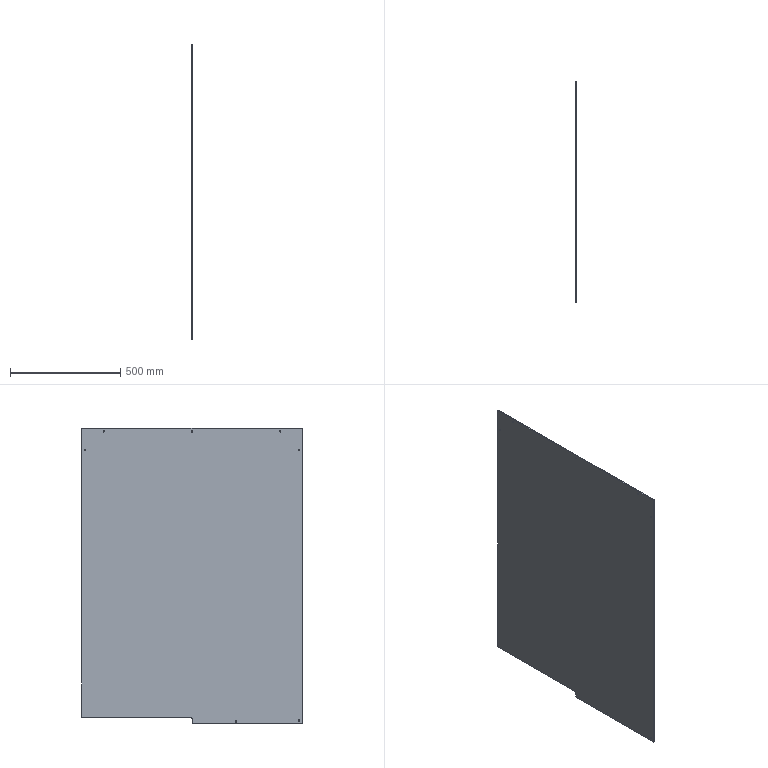Part | SolidWorks | features Chamfer 2, Fillet 2, ICE 2, Extrusion 1 | 1 solid | 28 faces | box 5 x 1000 x 1340 mm | volume 6624000 mm3 | cylinder 16 | plane 12 | commonest cylinder face diameters 6 x14 10 x2
STEP:
#1=CARTESIAN_POINT('',(5.,-200.,-662.));
#2=VERTEX_POINT('',#1);
#3=CARTESIAN_POINT('',(5.,-200.,-656.));
#4=VERTEX_POINT('',#3);
#5=CARTESIAN_POINT('',(5.,-200.,-659.));
#6=DIRECTION('',(-1.,0.,0.));
#7=DIRECTION('',(0.,0.,1.));
#8=AXIS2_PLACEMENT_3D('',#5,#6,#7);
#9=CIRCLE('',#8,3.);
#10=EDGE_CURVE('',#2,#4,#9,.T.);
#11=ORIENTED_EDGE('',*,*,#10,.F.);
#12=CARTESIAN_POINT('',(0.,-200.,-662.));
#13=VERTEX_POINT('',#12);
#14=CARTESIAN_POINT('',(5.,-200.,-662.));
#15=DIRECTION('',(-1.,0.,0.));
#16=VECTOR('',#15,1000.);
#17=LINE('',#14,#16);
#18=EDGE_CURVE('',#2,#13,#17,.T.);
#19=ORIENTED_EDGE('',*,*,#18,.T.);
#20=CARTESIAN_POINT('',(0.,-200.,-656.));
#21=VERTEX_POINT('',#20);
#22=CARTESIAN_POINT('',(0.,-200.,-659.));
#23=DIRECTION('',(-1.,0.,0.));
#24=DIRECTION('',(0.,0.,1.));
#25=AXIS2_PLACEMENT_3D('',#22,#23,#24);
#26=CIRCLE('',#25,3.);
#27=EDGE_CURVE('',#13,#21,#26,.T.);
#28=ORIENTED_EDGE('',*,*,#27,.T.);
#29=CARTESIAN_POINT('',(5.,-200.,-656.));
#30=DIRECTION('',(-1.,0.,0.));
#31=VECTOR('',#30,1000.);
#32=LINE('',#29,#31);
#33=EDGE_CURVE('',#4,#21,#32,.T.);
#34=ORIENTED_EDGE('',*,*,#33,.F.);
#35=EDGE_LOOP('',(#11,#19,#28,#34));
#36=FACE_OUTER_BOUND('',#35,.T.);
#37=CARTESIAN_POINT('',(5.,-200.,-659.));
#38=DIRECTION('',(-1.,0.,0.));
#39=DIRECTION('',(0.,0.,1.));
#40=AXIS2_PLACEMENT_3D('',#37,#38,#39);
#41=CYLINDRICAL_SURFACE('',#40,3.);
#42=ADVANCED_FACE('',(#36),#41,.F.);
#43=CARTESIAN_POINT('',(5.,0.,652.));
#44=VERTEX_POINT('',#43);
#45=CARTESIAN_POINT('',(5.,0.,658.));
#46=VERTEX_POINT('',#45);
#47=CARTESIAN_POINT('',(5.,0.,655.));
#48=DIRECTION('',(-1.,0.,0.));
#49=DIRECTION('',(0.,0.,1.));
#50=AXIS2_PLACEMENT_3D('',#47,#48,#49);
#51=CIRCLE('',#50,3.);
#52=EDGE_CURVE('',#44,#46,#51,.T.);
#53=ORIENTED_EDGE('',*,*,#52,.F.);
#54=CARTESIAN_POINT('',(0.,0.,652.));
#55=VERTEX_POINT('',#54);
#56=CARTESIAN_POINT('',(5.,0.,652.));
#57=DIRECTION('',(-1.,0.,0.));
#58=VECTOR('',#57,1000.);
#59=LINE('',#56,#58);
#60=EDGE_CURVE('',#44,#55,#59,.T.);
#61=ORIENTED_EDGE('',*,*,#60,.T.);
#62=CARTESIAN_POINT('',(0.,0.,658.));
#63=VERTEX_POINT('',#62);
#64=CARTESIAN_POINT('',(0.,0.,655.));
#65=DIRECTION('',(-1.,0.,0.));
#66=DIRECTION('',(0.,0.,1.));
#67=AXIS2_PLACEMENT_3D('',#64,#65,#66);
#68=CIRCLE('',#67,3.);
#69=EDGE_CURVE('',#55,#63,#68,.T.);
#70=ORIENTED_EDGE('',*,*,#69,.T.);
#71=CARTESIAN_POINT('',(5.,0.,658.));
#72=DIRECTION('',(-1.,0.,0.));
#73=VECTOR('',#72,1000.);
#74=LINE('',#71,#73);
#75=EDGE_CURVE('',#46,#63,#74,.T.);
#76=ORIENTED_EDGE('',*,*,#75,.F.);
#77=EDGE_LOOP('',(#53,#61,#70,#76));
#78=FACE_OUTER_BOUND('',#77,.T.);
#79=CARTESIAN_POINT('',(5.,0.,655.));
#80=DIRECTION('',(-1.,0.,0.));
#81=DIRECTION('',(0.,0.,1.));
#82=AXIS2_PLACEMENT_3D('',#79,#80,#81);
#83=CYLINDRICAL_SURFACE('',#82,3.);
#84=ADVANCED_FACE('',(#78),#83,.F.);
#85=CARTESIAN_POINT('',(5.,-485.,567.));
#86=VERTEX_POINT('',#85);
#87=CARTESIAN_POINT('',(5.,-485.,573.));
#88=VERTEX_POINT('',#87);
#89=CARTESIAN_POINT('',(5.,-485.,570.));
#90=DIRECTION('',(-1.,0.,0.));
#91=DIRECTION('',(0.,0.,1.));
#92=AXIS2_PLACEMENT_3D('',#89,#90,#91);
#93=CIRCLE('',#92,3.);
#94=EDGE_CURVE('',#86,#88,#93,.T.);
#95=ORIENTED_EDGE('',*,*,#94,.F.);
#96=CARTESIAN_POINT('',(0.,-485.,567.));
#97=VERTEX_POINT('',#96);
#98=CARTESIAN_POINT('',(5.,-485.,567.));
#99=DIRECTION('',(-1.,0.,0.));
#100=VECTOR('',#99,1000.);
#101=LINE('',#98,#100);
#102=EDGE_CURVE('',#86,#97,#101,.T.);
#103=ORIENTED_EDGE('',*,*,#102,.T.);
#104=CARTESIAN_POINT('',(0.,-485.,573.));
#105=VERTEX_POINT('',#104);
#106=CARTESIAN_POINT('',(0.,-485.,570.));
#107=DIRECTION('',(-1.,0.,0.));
#108=DIRECTION('',(0.,0.,1.));
#109=AXIS2_PLACEMENT_3D('',#106,#107,#108);
#110=CIRCLE('',#109,3.);
#111=EDGE_CURVE('',#97,#105,#110,.T.);
#112=ORIENTED_EDGE('',*,*,#111,.T.);
#113=CARTESIAN_POINT('',(5.,-485.,573.));
#114=DIRECTION('',(-1.,0.,0.));
#115=VECTOR('',#114,1000.);
#116=LINE('',#113,#115);
#117=EDGE_CURVE('',#88,#105,#116,.T.);
#118=ORIENTED_EDGE('',*,*,#117,.F.);
#119=EDGE_LOOP('',(#95,#103,#112,#118));
#120=FACE_OUTER_BOUND('',#119,.T.);
#121=CARTESIAN_POINT('',(5.,-485.,570.));
#122=DIRECTION('',(-1.,0.,0.));
#123=DIRECTION('',(0.,0.,1.));
#124=AXIS2_PLACEMENT_3D('',#121,#122,#123);
#125=CYLINDRICAL_SURFACE('',#124,3.);
#126=ADVANCED_FACE('',(#120),#125,.F.);
#127=CARTESIAN_POINT('',(5.,-400.,652.));
#128=VERTEX_POINT('',#127);
#129=CARTESIAN_POINT('',(5.,-400.,658.));
#130=VERTEX_POINT('',#129);
#131=CARTESIAN_POINT('',(5.,-400.,655.));
#132=DIRECTION('',(-1.,0.,0.));
#133=DIRECTION('',(0.,0.,1.));
#134=AXIS2_PLACEMENT_3D('',#131,#132,#133);
#135=CIRCLE('',#134,3.);
#136=EDGE_CURVE('',#128,#130,#135,.T.);
#137=ORIENTED_EDGE('',*,*,#136,.F.);
#138=CARTESIAN_POINT('',(0.,-400.,652.));
#139=VERTEX_POINT('',#138);
#140=CARTESIAN_POINT('',(5.,-400.,652.));
#141=DIRECTION('',(-1.,0.,0.));
#142=VECTOR('',#141,1000.);
#143=LINE('',#140,#142);
#144=EDGE_CURVE('',#128,#139,#143,.T.);
#145=ORIENTED_EDGE('',*,*,#144,.T.);
#146=CARTESIAN_POINT('',(0.,-400.,658.));
#147=VERTEX_POINT('',#146);
#148=CARTESIAN_POINT('',(0.,-400.,655.));
#149=DIRECTION('',(-1.,0.,0.));
#150=DIRECTION('',(0.,0.,1.));
#151=AXIS2_PLACEMENT_3D('',#148,#149,#150);
#152=CIRCLE('',#151,3.);
#153=EDGE_CURVE('',#139,#147,#152,.T.);
#154=ORIENTED_EDGE('',*,*,#153,.T.);
#155=CARTESIAN_POINT('',(5.,-400.,658.));
#156=DIRECTION('',(-1.,0.,0.));
#157=VECTOR('',#156,1000.);
#158=LINE('',#155,#157);
#159=EDGE_CURVE('',#130,#147,#158,.T.);
#160=ORIENTED_EDGE('',*,*,#159,.F.);
#161=EDGE_LOOP('',(#137,#145,#154,#160));
#162=FACE_OUTER_BOUND('',#161,.T.);
#163=CARTESIAN_POINT('',(5.,-400.,655.));
#164=DIRECTION('',(-1.,0.,0.));
#165=DIRECTION('',(0.,0.,1.));
#166=AXIS2_PLACEMENT_3D('',#163,#164,#165);
#167=CYLINDRICAL_SURFACE('',#166,3.);
#168=ADVANCED_FACE('',(#162),#167,.F.);
#169=CARTESIAN_POINT('',(5.,400.,652.));
#170=VERTEX_POINT('',#169);
#171=CARTESIAN_POINT('',(5.,400.,658.));
#172=VERTEX_POINT('',#171);
#173=CARTESIAN_POINT('',(5.,400.,655.));
#174=DIRECTION('',(-1.,0.,0.));
#175=DIRECTION('',(0.,0.,1.));
#176=AXIS2_PLACEMENT_3D('',#173,#174,#175);
#177=CIRCLE('',#176,3.);
#178=EDGE_CURVE('',#170,#172,#177,.T.);
#179=ORIENTED_EDGE('',*,*,#178,.F.);
#180=CARTESIAN_POINT('',(0.,400.,652.));
#181=VERTEX_POINT('',#180);
#182=CARTESIAN_POINT('',(5.,400.,652.));
#183=DIRECTION('',(-1.,0.,0.));
#184=VECTOR('',#183,1000.);
#185=LINE('',#182,#184);
#186=EDGE_CURVE('',#170,#181,#185,.T.);
#187=ORIENTED_EDGE('',*,*,#186,.T.);
#188=CARTESIAN_POINT('',(0.,400.,658.));
#189=VERTEX_POINT('',#188);
#190=CARTESIAN_POINT('',(0.,400.,655.));
#191=DIRECTION('',(-1.,0.,0.));
#192=DIRECTION('',(0.,0.,1.));
#193=AXIS2_PLACEMENT_3D('',#190,#191,#192);
#194=CIRCLE('',#193,3.);
#195=EDGE_CURVE('',#181,#189,#194,.T.);
#196=ORIENTED_EDGE('',*,*,#195,.T.);
#197=CARTESIAN_POINT('',(5.,400.,658.));
#198=DIRECTION('',(-1.,0.,0.));
#199=VECTOR('',#198,1000.);
#200=LINE('',#197,#199);
#201=EDGE_CURVE('',#172,#189,#200,.T.);
#202=ORIENTED_EDGE('',*,*,#201,.F.);
#203=EDGE_LOOP('',(#179,#187,#196,#202));
#204=FACE_OUTER_BOUND('',#203,.T.);
#205=CARTESIAN_POINT('',(5.,400.,655.));
#206=DIRECTION('',(-1.,0.,0.));
#207=DIRECTION('',(0.,0.,1.));
#208=AXIS2_PLACEMENT_3D('',#205,#206,#207);
#209=CYLINDRICAL_SURFACE('',#208,3.);
#210=ADVANCED_FACE('',(#204),#209,.F.);
#211=CARTESIAN_POINT('',(5.,485.,567.));
#212=VERTEX_POINT('',#211);
#213=CARTESIAN_POINT('',(5.,485.,573.));
#214=VERTEX_POINT('',#213);
#215=CARTESIAN_POINT('',(5.,485.,570.));
#216=DIRECTION('',(-1.,0.,0.));
#217=DIRECTION('',(0.,0.,1.));
#218=AXIS2_PLACEMENT_3D('',#215,#216,#217);
#219=CIRCLE('',#218,3.);
#220=EDGE_CURVE('',#212,#214,#219,.T.);
#221=ORIENTED_EDGE('',*,*,#220,.F.);
#222=CARTESIAN_POINT('',(0.,485.,567.));
#223=VERTEX_POINT('',#222);
#224=CARTESIAN_POINT('',(5.,485.,567.));
#225=DIRECTION('',(-1.,0.,0.));
#226=VECTOR('',#225,1000.);
#227=LINE('',#224,#226);
#228=EDGE_CURVE('',#212,#223,#227,.T.);
#229=ORIENTED_EDGE('',*,*,#228,.T.);
#230=CARTESIAN_POINT('',(0.,485.,573.));
#231=VERTEX_POINT('',#230);
#232=CARTESIAN_POINT('',(0.,485.,570.));
#233=DIRECTION('',(-1.,0.,0.));
#234=DIRECTION('',(0.,0.,1.));
#235=AXIS2_PLACEMENT_3D('',#232,#233,#234);
#236=CIRCLE('',#235,3.);
#237=EDGE_CURVE('',#223,#231,#236,.T.);
#238=ORIENTED_EDGE('',*,*,#237,.T.);
#239=CARTESIAN_POINT('',(5.,485.,573.));
#240=DIRECTION('',(-1.,0.,0.));
#241=VECTOR('',#240,1000.);
#242=LINE('',#239,#241);
#243=EDGE_CURVE('',#214,#231,#242,.T.);
#244=ORIENTED_EDGE('',*,*,#243,.F.);
#245=EDGE_LOOP('',(#221,#229,#238,#244));
#246=FACE_OUTER_BOUND('',#245,.T.);
#247=CARTESIAN_POINT('',(5.,485.,570.));
#248=DIRECTION('',(-1.,0.,0.));
#249=DIRECTION('',(0.,0.,1.));
#250=AXIS2_PLACEMENT_3D('',#247,#248,#249);
#251=CYLINDRICAL_SURFACE('',#250,3.);
#252=ADVANCED_FACE('',(#246),#251,.F.);
#253=CARTESIAN_POINT('',(5.,-485.,-658.));
#254=VERTEX_POINT('',#253);
#255=CARTESIAN_POINT('',(5.,-485.,-652.));
#256=VERTEX_POINT('',#255);
#257=CARTESIAN_POINT('',(5.,-485.,-655.));
#258=DIRECTION('',(-1.,0.,0.));
#259=DIRECTION('',(0.,0.,-1.));
#260=AXIS2_PLACEMENT_3D('',#257,#258,#259);
#261=CIRCLE('',#260,3.);
#262=EDGE_CURVE('',#254,#256,#261,.T.);
#263=ORIENTED_EDGE('',*,*,#262,.F.);
#264=CARTESIAN_POINT('',(0.,-485.,-658.));
#265=VERTEX_POINT('',#264);
#266=CARTESIAN_POINT('',(5.,-485.,-658.));
#267=DIRECTION('',(-1.,0.,0.));
#268=VECTOR('',#267,1000.);
#269=LINE('',#266,#268);
#270=EDGE_CURVE('',#254,#265,#269,.T.);
#271=ORIENTED_EDGE('',*,*,#270,.T.);
#272=CARTESIAN_POINT('',(0.,-485.,-652.));
#273=VERTEX_POINT('',#272);
#274=CARTESIAN_POINT('',(0.,-485.,-655.));
#275=DIRECTION('',(-1.,0.,0.));
#276=DIRECTION('',(0.,0.,-1.));
#277=AXIS2_PLACEMENT_3D('',#274,#275,#276);
#278=CIRCLE('',#277,3.);
#279=EDGE_CURVE('',#265,#273,#278,.T.);
#280=ORIENTED_EDGE('',*,*,#279,.T.);
#281=CARTESIAN_POINT('',(5.,-485.,-652.));
#282=DIRECTION('',(-1.,0.,0.));
#283=VECTOR('',#282,1000.);
#284=LINE('',#281,#283);
#285=EDGE_CURVE('',#256,#273,#284,.T.);
#286=ORIENTED_EDGE('',*,*,#285,.F.);
#287=EDGE_LOOP('',(#263,#271,#280,#286));
#288=FACE_OUTER_BOUND('',#287,.T.);
#289=CARTESIAN_POINT('',(5.,-485.,-655.));
#290=DIRECTION('',(-1.,0.,0.));
#291=DIRECTION('',(0.,0.,1.));
#292=AXIS2_PLACEMENT_3D('',#289,#290,#291);
#293=CYLINDRICAL_SURFACE('',#292,3.);
#294=ADVANCED_FACE('',(#288),#293,.F.);
#295=CARTESIAN_POINT('',(0.,499.,670.));
#296=VERTEX_POINT('',#295);
#297=CARTESIAN_POINT('',(0.,-499.,670.));
#298=VERTEX_POINT('',#297);
#299=CARTESIAN_POINT('',(0.,500.,670.));
#300=DIRECTION('',(0.,-1.,0.));
#301=VECTOR('',#300,1000.);
#302=LINE('',#299,#301);
#303=EDGE_CURVE('',#296,#298,#302,.T.);
#304=ORIENTED_EDGE('',*,*,#303,.T.);
#305=CARTESIAN_POINT('',(5.,-499.,670.));
#306=VERTEX_POINT('',#305);
#307=CARTESIAN_POINT('',(5.,-499.,670.));
#308=DIRECTION('',(1.,0.,0.));
#309=VECTOR('',#308,1000.);
#310=LINE('',#307,#309);
#311=EDGE_CURVE('',#298,#306,#310,.T.);
#312=ORIENTED_EDGE('',*,*,#311,.T.);
#313=CARTESIAN_POINT('',(5.,499.,670.));
#314=VERTEX_POINT('',#313);
#315=CARTESIAN_POINT('',(5.,500.,670.));
#316=DIRECTION('',(0.,-1.,0.));
#317=VECTOR('',#316,1000.);
#318=LINE('',#315,#317);
#319=EDGE_CURVE('',#314,#306,#318,.T.);
#320=ORIENTED_EDGE('',*,*,#319,.F.);
#321=CARTESIAN_POINT('',(5.,499.,670.));
#322=DIRECTION('',(-1.,0.,0.));
#323=VECTOR('',#322,1000.);
#324=LINE('',#321,#323);
#325=EDGE_CURVE('',#314,#296,#324,.T.);
#326=ORIENTED_EDGE('',*,*,#325,.T.);
#327=EDGE_LOOP('',(#304,#312,#320,#326));
#328=FACE_OUTER_BOUND('',#327,.T.);
#329=CARTESIAN_POINT('',(5.,500.,670.));
#330=DIRECTION('',(0.,0.,-1.));
#331=DIRECTION('',(0.,1.,0.));
#332=AXIS2_PLACEMENT_3D('',#329,#330,#331);
#333=PLANE('',#332);
#334=ADVANCED_FACE('',(#328),#333,.F.);
#335=CARTESIAN_POINT('',(0.,-500.,669.));
#336=VERTEX_POINT('',#335);
#337=CARTESIAN_POINT('',(0.,-500.,-669.));
#338=VERTEX_POINT('',#337);
#339=CARTESIAN_POINT('',(0.,-500.,-670.));
#340=DIRECTION('',(0.,0.,-1.));
#341=VECTOR('',#340,1000.);
#342=LINE('',#339,#341);
#343=EDGE_CURVE('',#336,#338,#342,.T.);
#344=ORIENTED_EDGE('',*,*,#343,.T.);
#345=CARTESIAN_POINT('',(5.,-500.,-669.));
#346=VERTEX_POINT('',#345);
#347=CARTESIAN_POINT('',(5.,-500.,-669.));
#348=DIRECTION('',(1.,0.,0.));
#349=VECTOR('',#348,1000.);
#350=LINE('',#347,#349);
#351=EDGE_CURVE('',#338,#346,#350,.T.);
#352=ORIENTED_EDGE('',*,*,#351,.T.);
#353=CARTESIAN_POINT('',(5.,-500.,669.));
#354=VERTEX_POINT('',#353);
#355=CARTESIAN_POINT('',(5.,-500.,-670.));
#356=DIRECTION('',(0.,0.,-1.));
#357=VECTOR('',#356,1000.);
#358=LINE('',#355,#357);
#359=EDGE_CURVE('',#354,#346,#358,.T.);
#360=ORIENTED_EDGE('',*,*,#359,.F.);
#361=CARTESIAN_POINT('',(5.,-500.,669.));
#362=DIRECTION('',(-1.,0.,0.));
#363=VECTOR('',#362,1000.);
#364=LINE('',#361,#363);
#365=EDGE_CURVE('',#354,#336,#364,.T.);
#366=ORIENTED_EDGE('',*,*,#365,.T.);
#367=EDGE_LOOP('',(#344,#352,#360,#366));
#368=FACE_OUTER_BOUND('',#367,.T.);
#369=CARTESIAN_POINT('',(5.,-500.,-670.));
#370=DIRECTION('',(0.,1.,0.));
#371=DIRECTION('',(0.,0.,1.));
#372=AXIS2_PLACEMENT_3D('',#369,#370,#371);
#373=PLANE('',#372);
#374=ADVANCED_FACE('',(#368),#373,.F.);
#375=CARTESIAN_POINT('',(0.,-499.,-670.));
#376=VERTEX_POINT('',#375);
#377=CARTESIAN_POINT('',(0.,-5.,-670.));
#378=VERTEX_POINT('',#377);
#379=CARTESIAN_POINT('',(0.,500.,-670.));
#380=DIRECTION('',(0.,1.,0.));
#381=VECTOR('',#380,1000.);
#382=LINE('',#379,#381);
#383=EDGE_CURVE('',#376,#378,#382,.T.);
#384=ORIENTED_EDGE('',*,*,#383,.T.);
#385=CARTESIAN_POINT('',(5.,-5.,-670.));
#386=VERTEX_POINT('',#385);
#387=CARTESIAN_POINT('',(5.,-5.,-670.));
#388=DIRECTION('',(1.,0.,0.));
#389=VECTOR('',#388,1000.);
#390=LINE('',#387,#389);
#391=EDGE_CURVE('',#378,#386,#390,.T.);
#392=ORIENTED_EDGE('',*,*,#391,.T.);
#393=CARTESIAN_POINT('',(5.,-499.,-670.));
#394=VERTEX_POINT('',#393);
#395=CARTESIAN_POINT('',(5.,500.,-670.));
#396=DIRECTION('',(0.,1.,0.));
#397=VECTOR('',#396,1000.);
#398=LINE('',#395,#397);
#399=EDGE_CURVE('',#394,#386,#398,.T.);
#400=ORIENTED_EDGE('',*,*,#399,.F.);
#401=CARTESIAN_POINT('',(5.,-499.,-670.));
#402=DIRECTION('',(-1.,0.,0.));
#403=VECTOR('',#402,1000.);
#404=LINE('',#401,#403);
#405=EDGE_CURVE('',#394,#376,#404,.T.);
#406=ORIENTED_EDGE('',*,*,#405,.T.);
#407=EDGE_LOOP('',(#384,#392,#400,#406));
#408=FACE_OUTER_BOUND('',#407,.T.);
#409=CARTESIAN_POINT('',(5.,500.,-670.));
#410=DIRECTION('',(0.,0.,1.));
#411=DIRECTION('',(0.,-1.,0.));
#412=AXIS2_PLACEMENT_3D('',#409,#410,#411);
#413=PLANE('',#412);
#414=ADVANCED_FACE('',(#408),#413,.F.);
#415=CARTESIAN_POINT('',(5.,500.,-639.));
#416=VERTEX_POINT('',#415);
#417=CARTESIAN_POINT('',(5.,500.,669.));
#418=VERTEX_POINT('',#417);
#419=CARTESIAN_POINT('',(5.,500.,-670.));
#420=DIRECTION('',(0.,0.,1.));
#421=VECTOR('',#420,1000.);
#422=LINE('',#419,#421);
#423=EDGE_CURVE('',#416,#418,#422,.T.);
#424=ORIENTED_EDGE('',*,*,#423,.F.);
#425=CARTESIAN_POINT('',(0.,500.,-639.));
#426=VERTEX_POINT('',#425);
#427=CARTESIAN_POINT('',(5.,500.,-639.));
#428=DIRECTION('',(-1.,0.,0.));
#429=VECTOR('',#428,1000.);
#430=LINE('',#427,#429);
#431=EDGE_CURVE('',#416,#426,#430,.T.);
#432=ORIENTED_EDGE('',*,*,#431,.T.);
#433=CARTESIAN_POINT('',(0.,500.,669.));
#434=VERTEX_POINT('',#433);
#435=CARTESIAN_POINT('',(0.,500.,-670.));
#436=DIRECTION('',(0.,0.,1.));
#437=VECTOR('',#436,1000.);
#438=LINE('',#435,#437);
#439=EDGE_CURVE('',#426,#434,#438,.T.);
#440=ORIENTED_EDGE('',*,*,#439,.T.);
#441=CARTESIAN_POINT('',(5.,500.,669.));
#442=DIRECTION('',(1.,0.,0.));
#443=VECTOR('',#442,1000.);
#444=LINE('',#441,#443);
#445=EDGE_CURVE('',#434,#418,#444,.T.);
#446=ORIENTED_EDGE('',*,*,#445,.T.);
#447=EDGE_LOOP('',(#424,#432,#440,#446));
#448=FACE_OUTER_BOUND('',#447,.T.);
#449=CARTESIAN_POINT('',(5.,500.,-670.));
#450=DIRECTION('',(0.,-1.,0.));
#451=DIRECTION('',(0.,0.,-1.));
#452=AXIS2_PLACEMENT_3D('',#449,#450,#451);
#453=PLANE('',#452);
#454=ADVANCED_FACE('',(#448),#453,.F.);
#455=CARTESIAN_POINT('',(5.,-200.,-659.));
#456=DIRECTION('',(-1.,0.,0.));
#457=DIRECTION('',(0.,0.,1.));
#458=AXIS2_PLACEMENT_3D('',#455,#456,#457);
#459=CIRCLE('',#458,3.);
#460=EDGE_CURVE('',#4,#2,#459,.T.);
#461=ORIENTED_EDGE('',*,*,#460,.T.);
#462=ORIENTED_EDGE('',*,*,#10,.T.);
#463=EDGE_LOOP('',(#461,#462));
#464=FACE_BOUND('',#463,.T.);
#465=CARTESIAN_POINT('',(5.,0.,655.));
#466=DIRECTION('',(-1.,0.,0.));
#467=DIRECTION('',(0.,0.,1.));
#468=AXIS2_PLACEMENT_3D('',#465,#466,#467);
#469=CIRCLE('',#468,3.);
#470=EDGE_CURVE('',#46,#44,#469,.T.);
#471=ORIENTED_EDGE('',*,*,#470,.T.);
#472=ORIENTED_EDGE('',*,*,#52,.T.);
#473=EDGE_LOOP('',(#471,#472));
#474=FACE_BOUND('',#473,.T.);
#475=CARTESIAN_POINT('',(5.,-485.,570.));
#476=DIRECTION('',(-1.,0.,0.));
#477=DIRECTION('',(0.,0.,1.));
#478=AXIS2_PLACEMENT_3D('',#475,#476,#477);
#479=CIRCLE('',#478,3.);
#480=EDGE_CURVE('',#88,#86,#479,.T.);
#481=ORIENTED_EDGE('',*,*,#480,.T.);
#482=ORIENTED_EDGE('',*,*,#94,.T.);
#483=EDGE_LOOP('',(#481,#482));
#484=FACE_BOUND('',#483,.T.);
#485=CARTESIAN_POINT('',(5.,-400.,655.));
#486=DIRECTION('',(-1.,0.,0.));
#487=DIRECTION('',(0.,0.,1.));
#488=AXIS2_PLACEMENT_3D('',#485,#486,#487);
#489=CIRCLE('',#488,3.);
#490=EDGE_CURVE('',#130,#128,#489,.T.);
#491=ORIENTED_EDGE('',*,*,#490,.T.);
#492=ORIENTED_EDGE('',*,*,#136,.T.);
#493=EDGE_LOOP('',(#491,#492));
#494=FACE_BOUND('',#493,.T.);
#495=CARTESIAN_POINT('',(5.,400.,655.));
#496=DIRECTION('',(-1.,0.,0.));
#497=DIRECTION('',(0.,0.,1.));
#498=AXIS2_PLACEMENT_3D('',#495,#496,#497);
#499=CIRCLE('',#498,3.);
#500=EDGE_CURVE('',#172,#170,#499,.T.);
#501=ORIENTED_EDGE('',*,*,#500,.T.);
#502=ORIENTED_EDGE('',*,*,#178,.T.);
#503=EDGE_LOOP('',(#501,#502));
#504=FACE_BOUND('',#503,.T.);
#505=CARTESIAN_POINT('',(5.,485.,570.));
#506=DIRECTION('',(-1.,0.,0.));
#507=DIRECTION('',(0.,0.,1.));
#508=AXIS2_PLACEMENT_3D('',#505,#506,#507);
#509=CIRCLE('',#508,3.);
#510=EDGE_CURVE('',#214,#212,#509,.T.);
#511=ORIENTED_EDGE('',*,*,#510,.T.);
#512=ORIENTED_EDGE('',*,*,#220,.T.);
#513=EDGE_LOOP('',(#511,#512));
#514=FACE_BOUND('',#513,.T.);
#515=CARTESIAN_POINT('',(5.,-485.,-655.));
#516=DIRECTION('',(-1.,0.,0.));
#517=DIRECTION('',(0.,0.,-1.));
#518=AXIS2_PLACEMENT_3D('',#515,#516,#517);
#519=CIRCLE('',#518,3.);
#520=EDGE_CURVE('',#256,#254,#519,.T.);
#521=ORIENTED_EDGE('',*,*,#520,.T.);
#522=ORIENTED_EDGE('',*,*,#262,.T.);
#523=EDGE_LOOP('',(#521,#522));
#524=FACE_BOUND('',#523,.T.);
#525=ORIENTED_EDGE('',*,*,#399,.T.);
#526=CARTESIAN_POINT('',(5.,0.,-665.));
#527=VERTEX_POINT('',#526);
#528=CARTESIAN_POINT('',(5.,-5.,-665.));
#529=DIRECTION('',(1.,0.,0.));
#530=DIRECTION('',(0.,0.,1.));
#531=AXIS2_PLACEMENT_3D('',#528,#529,#530);
#532=CIRCLE('',#531,5.);
#533=EDGE_CURVE('',#386,#527,#532,.T.);
#534=ORIENTED_EDGE('',*,*,#533,.T.);
#535=CARTESIAN_POINT('',(5.,0.,-645.));
#536=VERTEX_POINT('',#535);
#537=CARTESIAN_POINT('',(5.,0.,-670.));
#538=DIRECTION('',(0.,0.,-1.));
#539=VECTOR('',#538,1000.);
#540=LINE('',#537,#539);
#541=EDGE_CURVE('',#536,#527,#540,.T.);
#542=ORIENTED_EDGE('',*,*,#541,.F.);
#543=CARTESIAN_POINT('',(5.,5.,-640.));
#544=VERTEX_POINT('',#543);
#545=CARTESIAN_POINT('',(5.,5.,-645.));
#546=DIRECTION('',(-1.,0.,0.));
#547=DIRECTION('',(0.,0.,1.));
#548=AXIS2_PLACEMENT_3D('',#545,#546,#547);
#549=CIRCLE('',#548,5.);
#550=EDGE_CURVE('',#536,#544,#549,.T.);
#551=ORIENTED_EDGE('',*,*,#550,.T.);
#552=CARTESIAN_POINT('',(5.,499.,-640.));
#553=VERTEX_POINT('',#552);
#554=CARTESIAN_POINT('',(5.,500.,-640.));
#555=DIRECTION('',(0.,-1.,0.));
#556=VECTOR('',#555,1000.);
#557=LINE('',#554,#556);
#558=EDGE_CURVE('',#553,#544,#557,.T.);
#559=ORIENTED_EDGE('',*,*,#558,.F.);
#560=CARTESIAN_POINT('',(5.,499.,-640.));
#561=DIRECTION('',(0.,0.7071,0.7071));
#562=VECTOR('',#561,1000.);
#563=LINE('',#560,#562);
#564=EDGE_CURVE('',#553,#416,#563,.T.);
#565=ORIENTED_EDGE('',*,*,#564,.T.);
#566=ORIENTED_EDGE('',*,*,#423,.T.);
#567=CARTESIAN_POINT('',(5.,499.,670.));
#568=DIRECTION('',(0.,-0.7071,0.7071));
#569=VECTOR('',#568,1000.);
#570=LINE('',#567,#569);
#571=EDGE_CURVE('',#418,#314,#570,.T.);
#572=ORIENTED_EDGE('',*,*,#571,.T.);
#573=ORIENTED_EDGE('',*,*,#319,.T.);
#574=CARTESIAN_POINT('',(5.,-500.,669.));
#575=DIRECTION('',(0.,-0.7071,-0.7071));
#576=VECTOR('',#575,1000.);
#577=LINE('',#574,#576);
#578=EDGE_CURVE('',#306,#354,#577,.T.);
#579=ORIENTED_EDGE('',*,*,#578,.T.);
#580=ORIENTED_EDGE('',*,*,#359,.T.);
#581=CARTESIAN_POINT('',(5.,-499.,-670.));
#582=DIRECTION('',(0.,0.7071,-0.7071));
#583=VECTOR('',#582,1000.);
#584=LINE('',#581,#583);
#585=EDGE_CURVE('',#346,#394,#584,.T.);
#586=ORIENTED_EDGE('',*,*,#585,.T.);
#587=EDGE_LOOP('',(#525,#534,#542,#551,#559,#565,#566,#572,#573,#579,#580,#586));
#588=FACE_OUTER_BOUND('',#587,.T.);
#589=CARTESIAN_POINT('',(5.,-500.,670.));
#590=DIRECTION('',(-1.,0.,0.));
#591=DIRECTION('',(0.,0.,1.));
#592=AXIS2_PLACEMENT_3D('',#589,#590,#591);
#593=PLANE('',#592);
#594=ADVANCED_FACE('',(#464,#474,#484,#494,#504,#514,#524,#588),#593,.F.);
#595=CARTESIAN_POINT('',(0.,0.,-665.));
#596=VERTEX_POINT('',#595);
#597=CARTESIAN_POINT('',(0.,0.,-645.));
#598=VERTEX_POINT('',#597);
#599=CARTESIAN_POINT('',(0.,0.,670.));
#600=DIRECTION('',(0.,0.,1.));
#601=VECTOR('',#600,1000.);
#602=LINE('',#599,#601);
#603=EDGE_CURVE('',#596,#598,#602,.T.);
#604=ORIENTED_EDGE('',*,*,#603,.F.);
#605=CARTESIAN_POINT('',(0.,-5.,-665.));
#606=DIRECTION('',(-1.,0.,0.));
#607=DIRECTION('',(0.,0.,1.));
#608=AXIS2_PLACEMENT_3D('',#605,#606,#607);
#609=CIRCLE('',#608,5.);
#610=EDGE_CURVE('',#596,#378,#609,.T.);
#611=ORIENTED_EDGE('',*,*,#610,.T.);
#612=ORIENTED_EDGE('',*,*,#383,.F.);
#613=CARTESIAN_POINT('',(0.,-1169.5,0.5));
#614=DIRECTION('',(0.,-0.7071,0.7071));
#615=VECTOR('',#614,1000.);
#616=LINE('',#613,#615);
#617=EDGE_CURVE('',#376,#338,#616,.T.);
#618=ORIENTED_EDGE('',*,*,#617,.T.);
#619=ORIENTED_EDGE('',*,*,#343,.F.);
#620=CARTESIAN_POINT('',(0.,-499.5,669.5));
#621=DIRECTION('',(0.,0.7071,0.7071));
#622=VECTOR('',#621,1000.);
#623=LINE('',#620,#622);
#624=EDGE_CURVE('',#336,#298,#623,.T.);
#625=ORIENTED_EDGE('',*,*,#624,.T.);
#626=ORIENTED_EDGE('',*,*,#303,.F.);
#627=CARTESIAN_POINT('',(0.,-0.5,1169.5));
#628=DIRECTION('',(0.,0.7071,-0.7071));
#629=VECTOR('',#628,1000.);
#630=LINE('',#627,#629);
#631=EDGE_CURVE('',#296,#434,#630,.T.);
#632=ORIENTED_EDGE('',*,*,#631,.T.);
#633=ORIENTED_EDGE('',*,*,#439,.F.);
#634=CARTESIAN_POINT('',(0.,499.,-640.));
#635=VERTEX_POINT('',#634);
#636=CARTESIAN_POINT('',(0.,654.5,-484.5));
#637=DIRECTION('',(0.,-0.7071,-0.7071));
#638=VECTOR('',#637,1000.);
#639=LINE('',#636,#638);
#640=EDGE_CURVE('',#426,#635,#639,.T.);
#641=ORIENTED_EDGE('',*,*,#640,.T.);
#642=CARTESIAN_POINT('',(0.,5.,-640.));
#643=VERTEX_POINT('',#642);
#644=CARTESIAN_POINT('',(0.,-500.,-640.));
#645=DIRECTION('',(0.,1.,0.));
#646=VECTOR('',#645,1000.);
#647=LINE('',#644,#646);
#648=EDGE_CURVE('',#643,#635,#647,.T.);
#649=ORIENTED_EDGE('',*,*,#648,.F.);
#650=CARTESIAN_POINT('',(0.,5.,-645.));
#651=DIRECTION('',(1.,0.,0.));
#652=DIRECTION('',(0.,0.,1.));
#653=AXIS2_PLACEMENT_3D('',#650,#651,#652);
#654=CIRCLE('',#653,5.);
#655=EDGE_CURVE('',#643,#598,#654,.T.);
#656=ORIENTED_EDGE('',*,*,#655,.T.);
#657=EDGE_LOOP('',(#604,#611,#612,#618,#619,#625,#626,#632,#633,#641,#649,#656));
#658=FACE_OUTER_BOUND('',#657,.T.);
#659=CARTESIAN_POINT('',(0.,-200.,-659.));
#660=DIRECTION('',(-1.,0.,0.));
#661=DIRECTION('',(0.,0.,1.));
#662=AXIS2_PLACEMENT_3D('',#659,#660,#661);
#663=CIRCLE('',#662,3.);
#664=EDGE_CURVE('',#21,#13,#663,.T.);
#665=ORIENTED_EDGE('',*,*,#664,.F.);
#666=ORIENTED_EDGE('',*,*,#27,.F.);
#667=EDGE_LOOP('',(#665,#666));
#668=FACE_BOUND('',#667,.T.);
#669=CARTESIAN_POINT('',(0.,0.,655.));
#670=DIRECTION('',(-1.,0.,0.));
#671=DIRECTION('',(0.,0.,1.));
#672=AXIS2_PLACEMENT_3D('',#669,#670,#671);
#673=CIRCLE('',#672,3.);
#674=EDGE_CURVE('',#63,#55,#673,.T.);
#675=ORIENTED_EDGE('',*,*,#674,.F.);
#676=ORIENTED_EDGE('',*,*,#69,.F.);
#677=EDGE_LOOP('',(#675,#676));
#678=FACE_BOUND('',#677,.T.);
#679=CARTESIAN_POINT('',(0.,-485.,570.));
#680=DIRECTION('',(-1.,0.,0.));
#681=DIRECTION('',(0.,0.,1.));
#682=AXIS2_PLACEMENT_3D('',#679,#680,#681);
#683=CIRCLE('',#682,3.);
#684=EDGE_CURVE('',#105,#97,#683,.T.);
#685=ORIENTED_EDGE('',*,*,#684,.F.);
#686=ORIENTED_EDGE('',*,*,#111,.F.);
#687=EDGE_LOOP('',(#685,#686));
#688=FACE_BOUND('',#687,.T.);
#689=CARTESIAN_POINT('',(0.,-400.,655.));
#690=DIRECTION('',(-1.,0.,0.));
#691=DIRECTION('',(0.,0.,1.));
#692=AXIS2_PLACEMENT_3D('',#689,#690,#691);
#693=CIRCLE('',#692,3.);
#694=EDGE_CURVE('',#147,#139,#693,.T.);
#695=ORIENTED_EDGE('',*,*,#694,.F.);
#696=ORIENTED_EDGE('',*,*,#153,.F.);
#697=EDGE_LOOP('',(#695,#696));
#698=FACE_BOUND('',#697,.T.);
#699=CARTESIAN_POINT('',(0.,400.,655.));
#700=DIRECTION('',(-1.,0.,0.));
#701=DIRECTION('',(0.,0.,1.));
#702=AXIS2_PLACEMENT_3D('',#699,#700,#701);
#703=CIRCLE('',#702,3.);
#704=EDGE_CURVE('',#189,#181,#703,.T.);
#705=ORIENTED_EDGE('',*,*,#704,.F.);
#706=ORIENTED_EDGE('',*,*,#195,.F.);
#707=EDGE_LOOP('',(#705,#706));
#708=FACE_BOUND('',#707,.T.);
#709=CARTESIAN_POINT('',(0.,485.,570.));
#710=DIRECTION('',(-1.,0.,0.));
#711=DIRECTION('',(0.,0.,1.));
#712=AXIS2_PLACEMENT_3D('',#709,#710,#711);
#713=CIRCLE('',#712,3.);
#714=EDGE_CURVE('',#231,#223,#713,.T.);
#715=ORIENTED_EDGE('',*,*,#714,.F.);
#716=ORIENTED_EDGE('',*,*,#237,.F.);
#717=EDGE_LOOP('',(#715,#716));
#718=FACE_BOUND('',#717,.T.);
#719=CARTESIAN_POINT('',(0.,-485.,-655.));
#720=DIRECTION('',(-1.,0.,0.));
#721=DIRECTION('',(0.,0.,-1.));
#722=AXIS2_PLACEMENT_3D('',#719,#720,#721);
#723=CIRCLE('',#722,3.);
#724=EDGE_CURVE('',#273,#265,#723,.T.);
#725=ORIENTED_EDGE('',*,*,#724,.F.);
#726=ORIENTED_EDGE('',*,*,#279,.F.);
#727=EDGE_LOOP('',(#725,#726));
#728=FACE_BOUND('',#727,.T.);
#729=CARTESIAN_POINT('',(0.,-500.,670.));
#730=DIRECTION('',(-1.,0.,0.));
#731=DIRECTION('',(0.,0.,1.));
#732=AXIS2_PLACEMENT_3D('',#729,#730,#731);
#733=PLANE('',#732);
#734=ADVANCED_FACE('',(#658,#668,#678,#688,#698,#708,#718,#728),#733,.T.);
#735=ORIENTED_EDGE('',*,*,#585,.F.);
#736=ORIENTED_EDGE('',*,*,#351,.F.);
#737=ORIENTED_EDGE('',*,*,#617,.F.);
#738=ORIENTED_EDGE('',*,*,#405,.F.);
#739=EDGE_LOOP('',(#735,#736,#737,#738));
#740=FACE_OUTER_BOUND('',#739,.T.);
#741=CARTESIAN_POINT('',(5.,-499.,-670.));
#742=DIRECTION('',(0.,0.7071,0.7071));
#743=DIRECTION('',(0.,-0.7071,0.7071));
#744=AXIS2_PLACEMENT_3D('',#741,#742,#743);
#745=PLANE('',#744);
#746=ADVANCED_FACE('',(#740),#745,.F.);
#747=ORIENTED_EDGE('',*,*,#578,.F.);
#748=ORIENTED_EDGE('',*,*,#311,.F.);
#749=ORIENTED_EDGE('',*,*,#624,.F.);
#750=ORIENTED_EDGE('',*,*,#365,.F.);
#751=EDGE_LOOP('',(#747,#748,#749,#750));
#752=FACE_OUTER_BOUND('',#751,.T.);
#753=CARTESIAN_POINT('',(5.,-500.,669.));
#754=DIRECTION('',(0.,0.7071,-0.7071));
#755=DIRECTION('',(0.,0.7071,0.7071));
#756=AXIS2_PLACEMENT_3D('',#753,#754,#755);
#757=PLANE('',#756);
#758=ADVANCED_FACE('',(#752),#757,.F.);
#759=ORIENTED_EDGE('',*,*,#571,.F.);
#760=ORIENTED_EDGE('',*,*,#445,.F.);
#761=ORIENTED_EDGE('',*,*,#631,.F.);
#762=ORIENTED_EDGE('',*,*,#325,.F.);
#763=EDGE_LOOP('',(#759,#760,#761,#762));
#764=FACE_OUTER_BOUND('',#763,.T.);
#765=CARTESIAN_POINT('',(5.,499.,670.));
#766=DIRECTION('',(0.,-0.7071,-0.7071));
#767=DIRECTION('',(0.,0.7071,-0.7071));
#768=AXIS2_PLACEMENT_3D('',#765,#766,#767);
#769=PLANE('',#768);
#770=ADVANCED_FACE('',(#764),#769,.F.);
#771=ORIENTED_EDGE('',*,*,#270,.F.);
#772=ORIENTED_EDGE('',*,*,#520,.F.);
#773=ORIENTED_EDGE('',*,*,#285,.T.);
#774=ORIENTED_EDGE('',*,*,#724,.T.);
#775=EDGE_LOOP('',(#771,#772,#773,#774));
#776=FACE_OUTER_BOUND('',#775,.T.);
#777=CARTESIAN_POINT('',(5.,-485.,-655.));
#778=DIRECTION('',(-1.,0.,0.));
#779=DIRECTION('',(0.,0.,1.));
#780=AXIS2_PLACEMENT_3D('',#777,#778,#779);
#781=CYLINDRICAL_SURFACE('',#780,3.);
#782=ADVANCED_FACE('',(#776),#781,.F.);
#783=ORIENTED_EDGE('',*,*,#228,.F.);
#784=ORIENTED_EDGE('',*,*,#510,.F.);
#785=ORIENTED_EDGE('',*,*,#243,.T.);
#786=ORIENTED_EDGE('',*,*,#714,.T.);
#787=EDGE_LOOP('',(#783,#784,#785,#786));
#788=FACE_OUTER_BOUND('',#787,.T.);
#789=CARTESIAN_POINT('',(5.,485.,570.));
#790=DIRECTION('',(-1.,0.,0.));
#791=DIRECTION('',(0.,0.,1.));
#792=AXIS2_PLACEMENT_3D('',#789,#790,#791);
#793=CYLINDRICAL_SURFACE('',#792,3.);
#794=ADVANCED_FACE('',(#788),#793,.F.);
#795=ORIENTED_EDGE('',*,*,#186,.F.);
#796=ORIENTED_EDGE('',*,*,#500,.F.);
#797=ORIENTED_EDGE('',*,*,#201,.T.);
#798=ORIENTED_EDGE('',*,*,#704,.T.);
#799=EDGE_LOOP('',(#795,#796,#797,#798));
#800=FACE_OUTER_BOUND('',#799,.T.);
#801=CARTESIAN_POINT('',(5.,400.,655.));
#802=DIRECTION('',(-1.,0.,0.));
#803=DIRECTION('',(0.,0.,1.));
#804=AXIS2_PLACEMENT_3D('',#801,#802,#803);
#805=CYLINDRICAL_SURFACE('',#804,3.);
#806=ADVANCED_FACE('',(#800),#805,.F.);
#807=ORIENTED_EDGE('',*,*,#144,.F.);
#808=ORIENTED_EDGE('',*,*,#490,.F.);
#809=ORIENTED_EDGE('',*,*,#159,.T.);
#810=ORIENTED_EDGE('',*,*,#694,.T.);
#811=EDGE_LOOP('',(#807,#808,#809,#810));
#812=FACE_OUTER_BOUND('',#811,.T.);
#813=CARTESIAN_POINT('',(5.,-400.,655.));
#814=DIRECTION('',(-1.,0.,0.));
#815=DIRECTION('',(0.,0.,1.));
#816=AXIS2_PLACEMENT_3D('',#813,#814,#815);
#817=CYLINDRICAL_SURFACE('',#816,3.);
#818=ADVANCED_FACE('',(#812),#817,.F.);
#819=ORIENTED_EDGE('',*,*,#102,.F.);
#820=ORIENTED_EDGE('',*,*,#480,.F.);
#821=ORIENTED_EDGE('',*,*,#117,.T.);
#822=ORIENTED_EDGE('',*,*,#684,.T.);
#823=EDGE_LOOP('',(#819,#820,#821,#822));
#824=FACE_OUTER_BOUND('',#823,.T.);
#825=CARTESIAN_POINT('',(5.,-485.,570.));
#826=DIRECTION('',(-1.,0.,0.));
#827=DIRECTION('',(0.,0.,1.));
#828=AXIS2_PLACEMENT_3D('',#825,#826,#827);
#829=CYLINDRICAL_SURFACE('',#828,3.);
#830=ADVANCED_FACE('',(#824),#829,.F.);
#831=ORIENTED_EDGE('',*,*,#60,.F.);
#832=ORIENTED_EDGE('',*,*,#470,.F.);
#833=ORIENTED_EDGE('',*,*,#75,.T.);
#834=ORIENTED_EDGE('',*,*,#674,.T.);
#835=EDGE_LOOP('',(#831,#832,#833,#834));
#836=FACE_OUTER_BOUND('',#835,.T.);
#837=CARTESIAN_POINT('',(5.,0.,655.));
#838=DIRECTION('',(-1.,0.,0.));
#839=DIRECTION('',(0.,0.,1.));
#840=AXIS2_PLACEMENT_3D('',#837,#838,#839);
#841=CYLINDRICAL_SURFACE('',#840,3.);
#842=ADVANCED_FACE('',(#836),#841,.F.);
#843=ORIENTED_EDGE('',*,*,#18,.F.);
#844=ORIENTED_EDGE('',*,*,#460,.F.);
#845=ORIENTED_EDGE('',*,*,#33,.T.);
#846=ORIENTED_EDGE('',*,*,#664,.T.);
#847=EDGE_LOOP('',(#843,#844,#845,#846));
#848=FACE_OUTER_BOUND('',#847,.T.);
#849=CARTESIAN_POINT('',(5.,-200.,-659.));
#850=DIRECTION('',(-1.,0.,0.));
#851=DIRECTION('',(0.,0.,1.));
#852=AXIS2_PLACEMENT_3D('',#849,#850,#851);
#853=CYLINDRICAL_SURFACE('',#852,3.);
#854=ADVANCED_FACE('',(#848),#853,.F.);
#855=ORIENTED_EDGE('',*,*,#541,.T.);
#856=CARTESIAN_POINT('',(-5.,0.,-665.));
#857=DIRECTION('',(-1.,0.,0.));
#858=VECTOR('',#857,1000.);
#859=LINE('',#856,#858);
#860=EDGE_CURVE('',#527,#596,#859,.T.);
#861=ORIENTED_EDGE('',*,*,#860,.T.);
#862=ORIENTED_EDGE('',*,*,#603,.T.);
#863=CARTESIAN_POINT('',(5.,0.,-645.));
#864=DIRECTION('',(1.,0.,0.));
#865=VECTOR('',#864,1000.);
#866=LINE('',#863,#865);
#867=EDGE_CURVE('',#598,#536,#866,.T.);
#868=ORIENTED_EDGE('',*,*,#867,.T.);
#869=EDGE_LOOP('',(#855,#861,#862,#868));
#870=FACE_OUTER_BOUND('',#869,.T.);
#871=CARTESIAN_POINT('',(-5.,0.,-670.));
#872=DIRECTION('',(0.,-1.,0.));
#873=DIRECTION('',(0.,0.,-1.));
#874=AXIS2_PLACEMENT_3D('',#871,#872,#873);
#875=PLANE('',#874);
#876=ADVANCED_FACE('',(#870),#875,.F.);
#877=ORIENTED_EDGE('',*,*,#558,.T.);
#878=CARTESIAN_POINT('',(0.,5.,-640.));
#879=DIRECTION('',(-1.,0.,0.));
#880=VECTOR('',#879,1000.);
#881=LINE('',#878,#880);
#882=EDGE_CURVE('',#544,#643,#881,.T.);
#883=ORIENTED_EDGE('',*,*,#882,.T.);
#884=ORIENTED_EDGE('',*,*,#648,.T.);
#885=CARTESIAN_POINT('',(-5.,499.,-640.));
#886=DIRECTION('',(1.,0.,0.));
#887=VECTOR('',#886,1000.);
#888=LINE('',#885,#887);
#889=EDGE_CURVE('',#635,#553,#888,.T.);
#890=ORIENTED_EDGE('',*,*,#889,.T.);
#891=EDGE_LOOP('',(#877,#883,#884,#890));
#892=FACE_OUTER_BOUND('',#891,.T.);
#893=CARTESIAN_POINT('',(-5.,500.,-640.));
#894=DIRECTION('',(0.,0.,1.));
#895=DIRECTION('',(1.,0.,0.));
#896=AXIS2_PLACEMENT_3D('',#893,#894,#895);
#897=PLANE('',#896);
#898=ADVANCED_FACE('',(#892),#897,.F.);
#899=ORIENTED_EDGE('',*,*,#640,.F.);
#900=ORIENTED_EDGE('',*,*,#431,.F.);
#901=ORIENTED_EDGE('',*,*,#564,.F.);
#902=ORIENTED_EDGE('',*,*,#889,.F.);
#903=EDGE_LOOP('',(#899,#900,#901,#902));
#904=FACE_OUTER_BOUND('',#903,.T.);
#905=CARTESIAN_POINT('',(-5.,499.,-640.));
#906=DIRECTION('',(0.,-0.7071,0.7071));
#907=DIRECTION('',(1.,0.,0.));
#908=AXIS2_PLACEMENT_3D('',#905,#906,#907);
#909=PLANE('',#908);
#910=ADVANCED_FACE('',(#904),#909,.F.);
#911=ORIENTED_EDGE('',*,*,#655,.F.);
#912=ORIENTED_EDGE('',*,*,#882,.F.);
#913=ORIENTED_EDGE('',*,*,#550,.F.);
#914=ORIENTED_EDGE('',*,*,#867,.F.);
#915=EDGE_LOOP('',(#911,#912,#913,#914));
#916=FACE_OUTER_BOUND('',#915,.T.);
#917=CARTESIAN_POINT('',(-5.,5.,-645.));
#918=DIRECTION('',(-1.,0.,0.));
#919=DIRECTION('',(0.,0.,1.));
#920=AXIS2_PLACEMENT_3D('',#917,#918,#919);
#921=CYLINDRICAL_SURFACE('',#920,5.);
#922=ADVANCED_FACE('',(#916),#921,.F.);
#923=ORIENTED_EDGE('',*,*,#610,.F.);
#924=ORIENTED_EDGE('',*,*,#860,.F.);
#925=ORIENTED_EDGE('',*,*,#533,.F.);
#926=ORIENTED_EDGE('',*,*,#391,.F.);
#927=EDGE_LOOP('',(#923,#924,#925,#926));
#928=FACE_OUTER_BOUND('',#927,.T.);
#929=CARTESIAN_POINT('',(5.,-5.,-665.));
#930=DIRECTION('',(1.,0.,0.));
#931=DIRECTION('',(0.,0.,-1.));
#932=AXIS2_PLACEMENT_3D('',#929,#930,#931);
#933=CYLINDRICAL_SURFACE('',#932,5.);
#934=ADVANCED_FACE('',(#928),#933,.T.);
#935=CLOSED_SHELL('',(#42,#84,#126,#168,#210,#252,#294,#334,#374,#414,#454,#594,#734,#746,#758,#770,#782,#794,#806,#818,#830,#842,#854,#876,#898,#910,#922,#934));
#936=MANIFOLD_SOLID_BREP('',#935);
#937=CARTESIAN_POINT('',(0.,0.,0.));
#938=DIRECTION('',(0.,0.,1.));
#939=DIRECTION('',(1.,0.,0.));
#940=AXIS2_PLACEMENT_3D('',#937,#938,#939);
#941=(LENGTH_UNIT()NAMED_UNIT(*)SI_UNIT(.MILLI.,.METRE.));
#942=UNCERTAINTY_MEASURE_WITH_UNIT(LENGTH_MEASURE(0.00001),#941,'','');
#943=(NAMED_UNIT(*)PLANE_ANGLE_UNIT()SI_UNIT($,.RADIAN.));
#944=(NAMED_UNIT(*)SI_UNIT($,.STERADIAN.)SOLID_ANGLE_UNIT());
#945=(GEOMETRIC_REPRESENTATION_CONTEXT(3)GLOBAL_UNCERTAINTY_ASSIGNED_CONTEXT((#942))GLOBAL_UNIT_ASSIGNED_CONTEXT((#941,#943,#944))REPRESENTATION_CONTEXT('',''));
#946=ADVANCED_BREP_SHAPE_REPRESENTATION('',(#936,#940),#945);